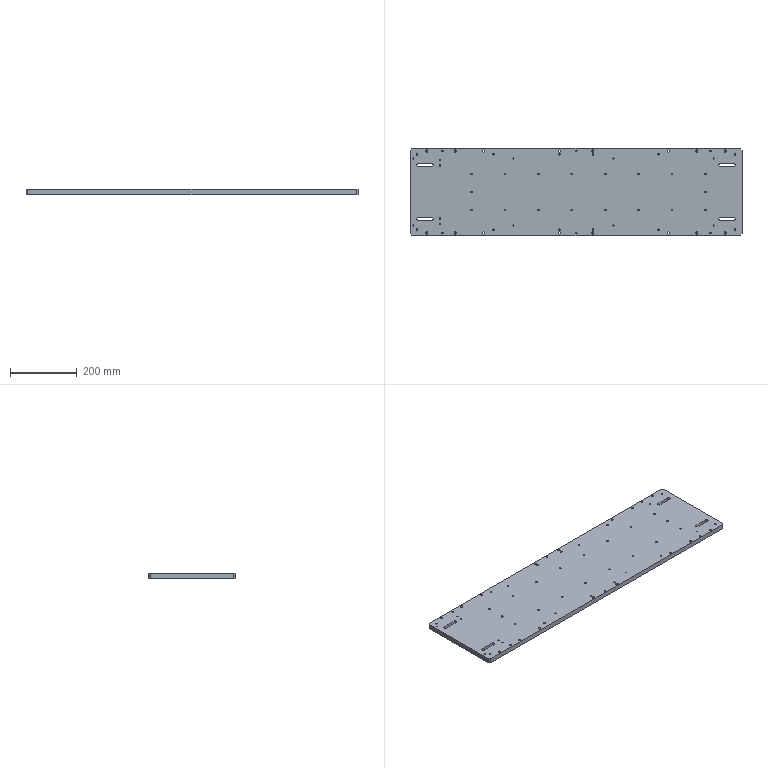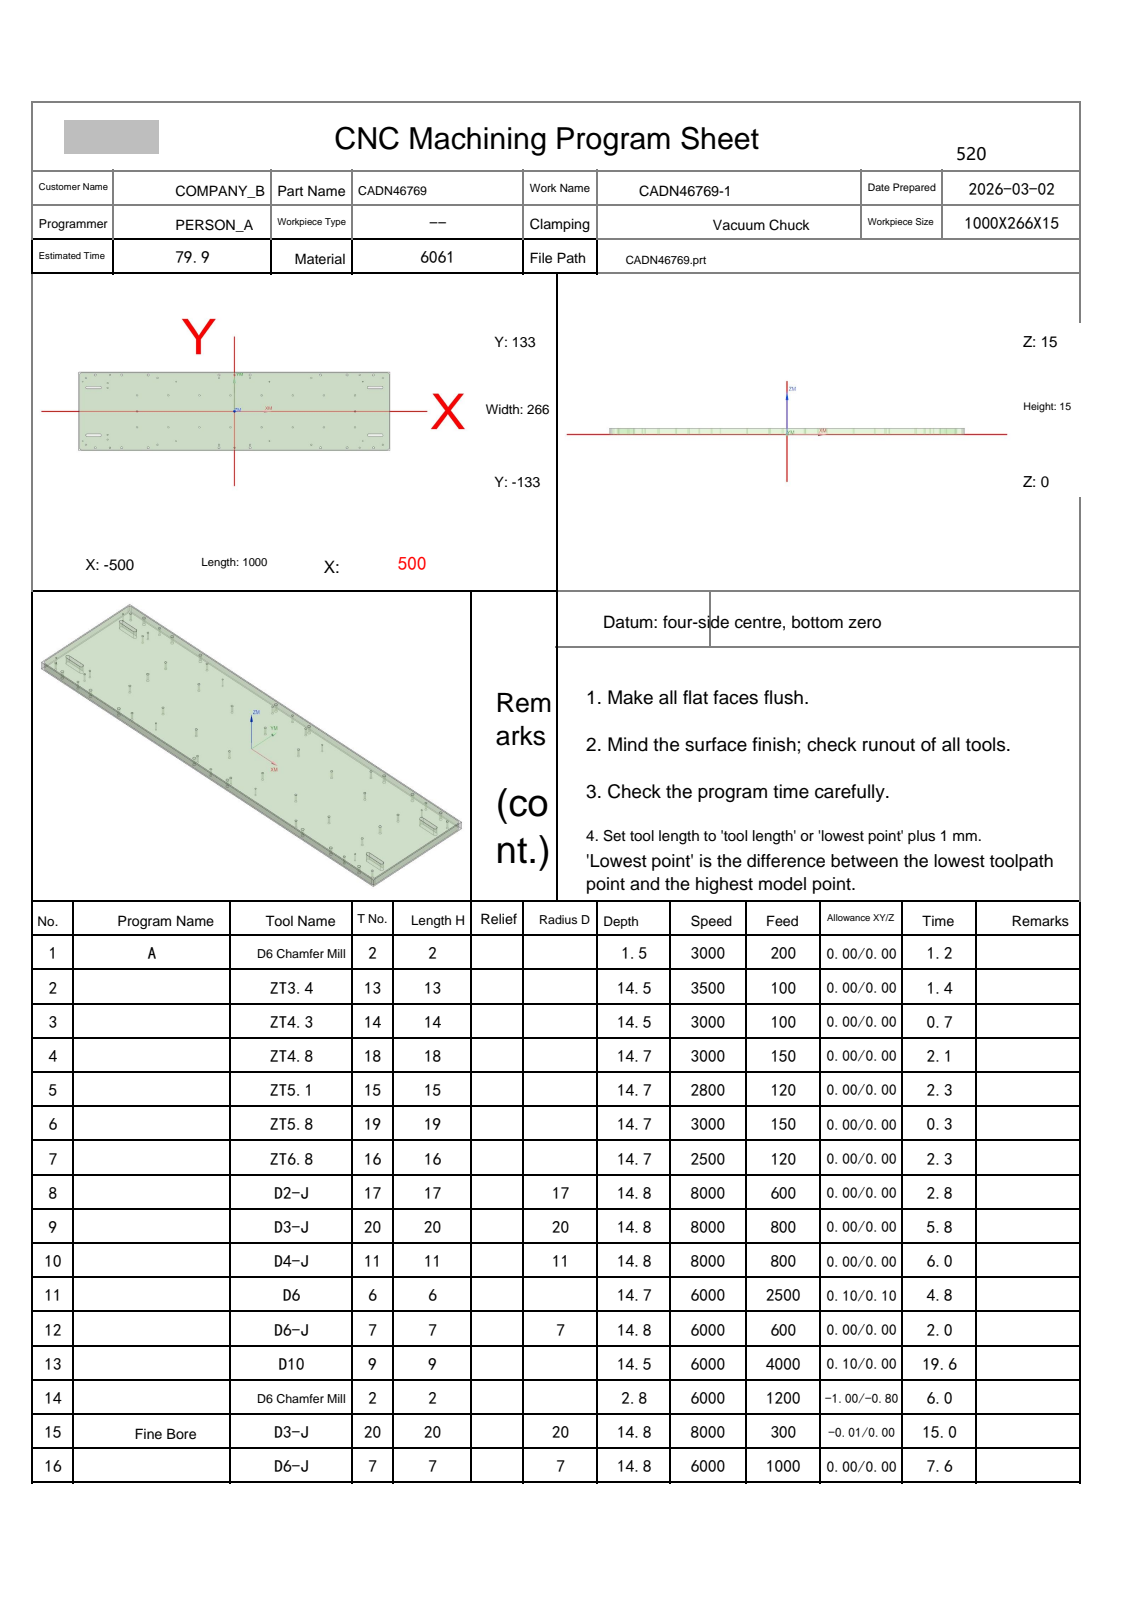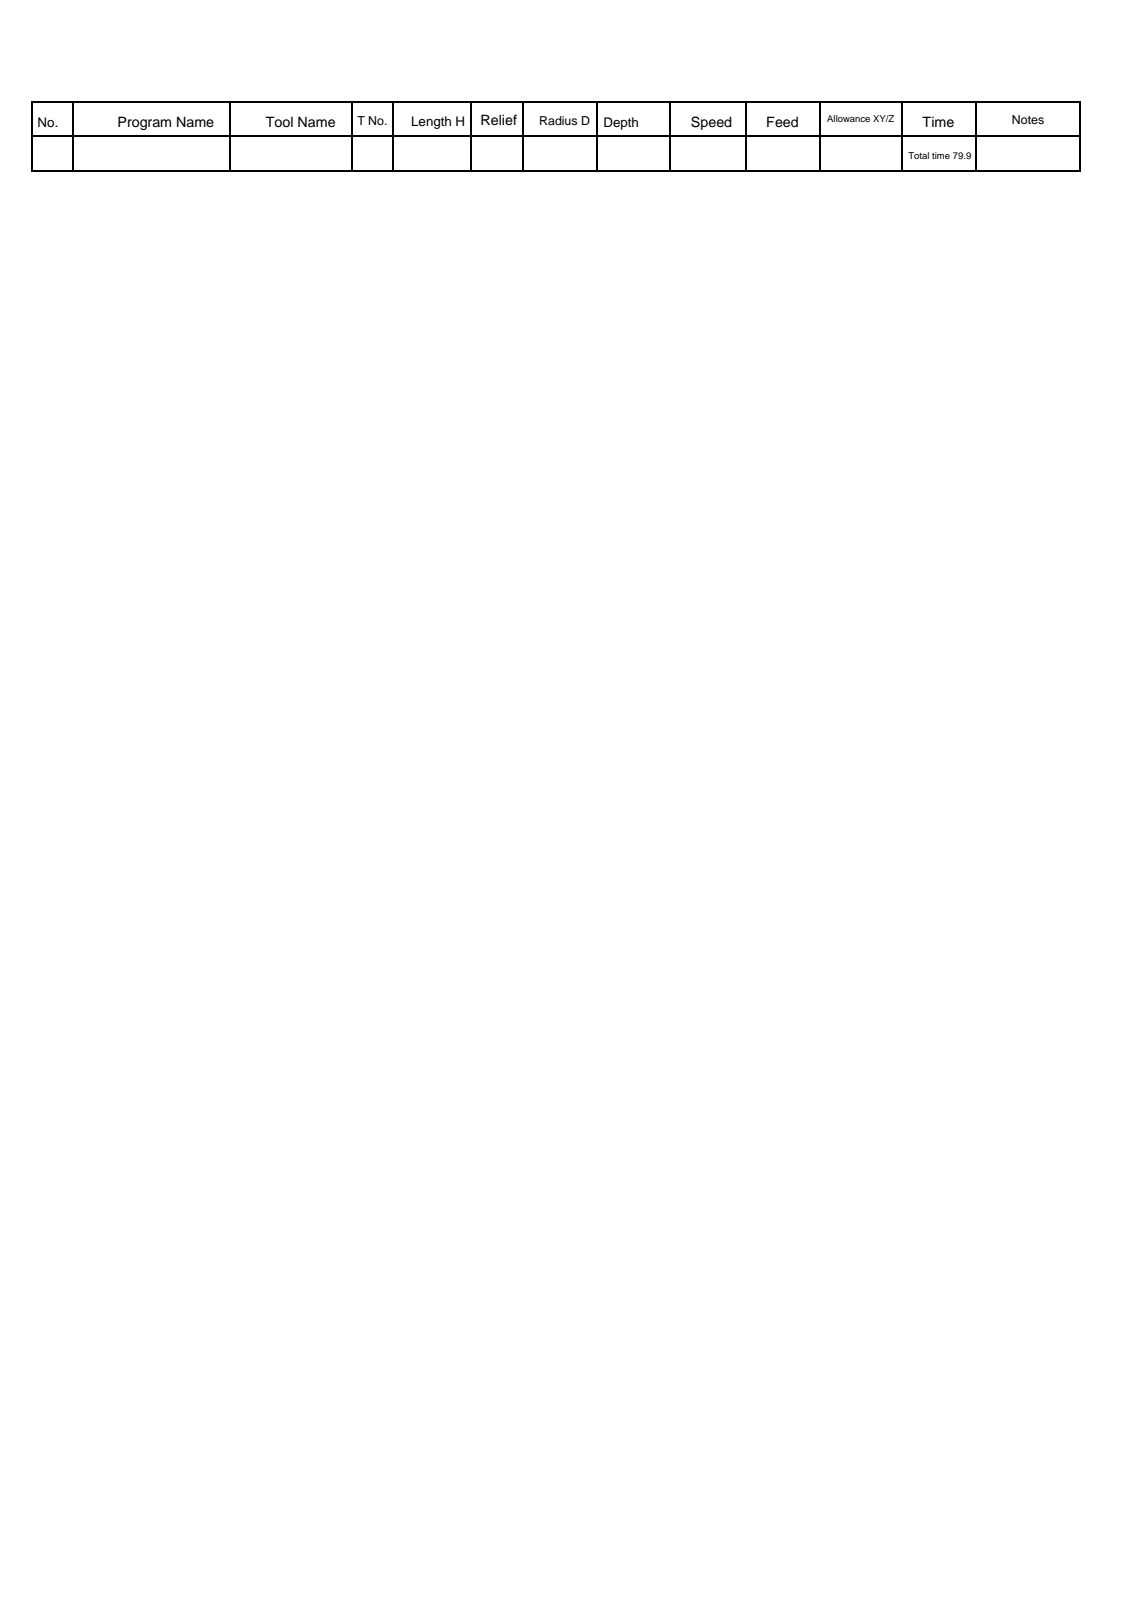NC program | NX | posted by the shop | part box 995 x 261 x 15 mm
Lines 2140 to 2975 of 14350:
N9 T20 M06
(D3-J  D=3. R=0. H=20 ce=0.00 di=0.00)
G00 G90 G54 X-407.387 Y-94.911 M03 S8000
G43 H20 Z45.
M08
Z15.5
G01 X-407.422 Y-94.9 Z15.498 F600.
X-407.578 Z15.49
X-407.767 Y-94.957 Z15.48
X-407.928 Y-95.072 Z15.469
X-408.043 Y-95.233 Z15.459
X-408.1 Y-95.422 Z15.448
Y-95.578 Z15.44
X-408.047 Y-95.758 Z15.43
X-407.941 Y-95.914 Z15.421
X-407.792 Y-96.03 Z15.411
X-407.615 Y-96.094 Z15.401
X-407.422 Y-96.1 Z15.391
X-407.233 Y-96.043 Z15.38
X-407.072 Y-95.928 Z15.37
X-406.957 Y-95.767 Z15.36
X-406.9 Y-95.578 Z15.349
Y-95.422 Z15.341
X-406.957 Y-95.233 Z15.331
X-407.072 Y-95.072 Z15.32
X-407.233 Y-94.957 Z15.31
X-407.422 Y-94.9 Z15.3
X-407.578 Z15.292
X-407.767 Y-94.957 Z15.281
X-407.928 Y-95.072 Z15.271
X-408.043 Y-95.233 Z15.26
X-408.1 Y-95.422 Z15.25
Y-95.578 Z15.242
X-408.047 Y-95.758 Z15.232
X-407.941 Y-95.914 Z15.222
X-407.792 Y-96.03 Z15.212
X-407.615 Y-96.094 Z15.202
X-407.422 Y-96.1 Z15.192
X-407.233 Y-96.043 Z15.182
X-407.072 Y-95.928 Z15.172
X-406.957 Y-95.767 Z15.161
X-406.9 Y-95.578 Z15.151
Y-95.422 Z15.143
X-406.957 Y-95.233 Z15.132
X-407.072 Y-95.072 Z15.122
X-407.233 Y-94.957 Z15.112
X-407.422 Y-94.9 Z15.101
X-407.578 Z15.093
X-407.767 Y-94.957 Z15.083
X-407.928 Y-95.072 Z15.072
X-408.043 Y-95.233 Z15.062
X-408.1 Y-95.422 Z15.052
Y-95.578 Z15.044
X-408.047 Y-95.758 Z15.034
X-407.941 Y-95.914 Z15.024
X-407.792 Y-96.03 Z15.014
X-407.615 Y-96.094 Z15.004
X-407.537 Y-96.099 Z15.
X-407.535 Y-96.065
G41 D20
X-407.5 Y-96.1
G03 X-406.9 Y-95.5 Z14.914 I0.0 J.6
X-407.5 Y-94.9 Z14.828 I-.6 J0.0
X-408.1 Y-95.5 Z14.742 I0.0 J-.6
X-407.5 Y-96.1 Z14.656 I.6 J0.0
X-406.9 Y-95.5 Z14.57 I0.0 J.6
X-407.5 Y-94.9 Z14.484 I-.6 J0.0
X-408.1 Y-95.5 Z14.398 I0.0 J-.6
X-407.5 Y-96.1 Z14.312 I.6 J0.0
X-406.9 Y-95.5 Z14.226 I0.0 J.6
X-407.5 Y-94.9 Z14.14 I-.6 J0.0
X-408.1 Y-95.5 Z14.053 I0.0 J-.6
X-407.5 Y-96.1 Z13.967 I.6 J0.0
X-406.9 Y-95.5 Z13.881 I0.0 J.6
X-407.5 Y-94.9 Z13.795 I-.6 J0.0
X-408.1 Y-95.5 Z13.709 I0.0 J-.6
X-407.5 Y-96.1 Z13.623 I.6 J0.0
X-406.9 Y-95.5 Z13.537 I0.0 J.6
X-407.5 Y-94.9 Z13.451 I-.6 J0.0
X-408.1 Y-95.5 Z13.365 I0.0 J-.6
X-407.5 Y-96.1 Z13.279 I.6 J0.0
X-406.9 Y-95.5 Z13.193 I0.0 J.6
X-407.5 Y-94.9 Z13.107 I-.6 J0.0
X-408.1 Y-95.5 Z13.021 I0.0 J-.6
X-407.5 Y-96.1 Z12.935 I.6 J0.0
X-406.9 Y-95.5 Z12.849 I0.0 J.6
X-407.5 Y-94.9 Z12.763 I-.6 J0.0
X-408.1 Y-95.5 Z12.677 I0.0 J-.6
X-407.5 Y-96.1 Z12.591 I.6 J0.0
X-406.9 Y-95.5 Z12.505 I0.0 J.6
X-407.5 Y-94.9 Z12.419 I-.6 J0.0
X-408.1 Y-95.5 Z12.333 I0.0 J-.6
X-407.5 Y-96.1 Z12.247 I.6 J0.0
X-406.9 Y-95.5 Z12.16 I0.0 J.6
X-407.5 Y-94.9 Z12.074 I-.6 J0.0
X-408.1 Y-95.5 Z11.988 I0.0 J-.6
X-407.5 Y-96.1 Z11.902 I.6 J0.0
X-406.9 Y-95.5 Z11.816 I0.0 J.6
X-407.5 Y-94.9 Z11.73 I-.6 J0.0
X-408.1 Y-95.5 Z11.644 I0.0 J-.6
X-407.5 Y-96.1 Z11.558 I.6 J0.0
X-406.9 Y-95.5 Z11.472 I0.0 J.6
X-407.5 Y-94.9 Z11.386 I-.6 J0.0
X-408.1 Y-95.5 Z11.3 I0.0 J-.6
X-407.5 Y-96.1 Z11.214 I.6 J0.0
X-406.9 Y-95.5 Z11.128 I0.0 J.6
X-407.5 Y-94.9 Z11.042 I-.6 J0.0
X-408.1 Y-95.5 Z10.956 I0.0 J-.6
X-407.5 Y-96.1 Z10.87 I.6 J0.0
X-406.9 Y-95.5 Z10.784 I0.0 J.6
X-407.5 Y-94.9 Z10.698 I-.6 J0.0
X-408.1 Y-95.5 Z10.612 I0.0 J-.6
X-407.5 Y-96.1 Z10.526 I.6 J0.0
X-406.9 Y-95.5 Z10.44 I0.0 J.6
X-407.5 Y-94.9 Z10.353 I-.6 J0.0
X-408.1 Y-95.5 Z10.267 I0.0 J-.6
X-407.5 Y-96.1 Z10.181 I.6 J0.0
X-406.9 Y-95.5 Z10.095 I0.0 J.6
X-407.5 Y-94.9 Z10.009 I-.6 J0.0
X-408.1 Y-95.5 Z9.923 I0.0 J-.6
X-407.5 Y-96.1 Z9.837 I.6 J0.0
X-406.9 Y-95.5 Z9.751 I0.0 J.6
X-407.5 Y-94.9 Z9.665 I-.6 J0.0
X-408.1 Y-95.5 Z9.579 I0.0 J-.6
X-407.5 Y-96.1 Z9.493 I.6 J0.0
X-406.9 Y-95.5 Z9.407 I0.0 J.6
X-407.5 Y-94.9 Z9.321 I-.6 J0.0
X-408.1 Y-95.5 Z9.235 I0.0 J-.6
X-407.5 Y-96.1 Z9.149 I.6 J0.0
X-406.9 Y-95.5 Z9.063 I0.0 J.6
X-407.5 Y-94.9 Z8.977 I-.6 J0.0
X-408.1 Y-95.5 Z8.891 I0.0 J-.6
X-407.5 Y-96.1 Z8.805 I.6 J0.0
X-406.9 Y-95.5 Z8.719 I0.0 J.6
X-407.5 Y-94.9 Z8.633 I-.6 J0.0
X-408.1 Y-95.5 Z8.547 I0.0 J-.6
X-407.5 Y-96.1 Z8.46 I.6 J0.0
X-406.9 Y-95.5 Z8.374 I0.0 J.6
X-407.5 Y-94.9 Z8.288 I-.6 J0.0
X-408.1 Y-95.5 Z8.202 I0.0 J-.6
X-407.5 Y-96.1 Z8.116 I.6 J0.0
X-406.9 Y-95.5 Z8.03 I0.0 J.6
X-407.5 Y-94.9 Z7.944 I-.6 J0.0
X-408.1 Y-95.5 Z7.858 I0.0 J-.6
X-407.5 Y-96.1 Z7.772 I.6 J0.0
X-406.9 Y-95.5 Z7.686 I0.0 J.6
X-407.5 Y-94.9 Z7.6 I-.6 J0.0
X-408.1 Y-95.5 Z7.514 I0.0 J-.6
X-407.5 Y-96.1 Z7.428 I.6 J0.0
X-406.9 Y-95.5 Z7.342 I0.0 J.6
X-407.5 Y-94.9 Z7.256 I-.6 J0.0
X-408.1 Y-95.5 Z7.17 I0.0 J-.6
X-407.5 Y-96.1 Z7.084 I.6 J0.0
X-406.9 Y-95.5 Z6.998 I0.0 J.6
X-407.5 Y-94.9 Z6.912 I-.6 J0.0
X-408.1 Y-95.5 Z6.826 I0.0 J-.6
X-407.5 Y-96.1 Z6.74 I.6 J0.0
X-406.9 Y-95.5 Z6.653 I0.0 J.6
X-407.5 Y-94.9 Z6.567 I-.6 J0.0
X-408.1 Y-95.5 Z6.481 I0.0 J-.6
X-407.5 Y-96.1 Z6.395 I.6 J0.0
X-406.9 Y-95.5 Z6.309 I0.0 J.6
X-407.5 Y-94.9 Z6.223 I-.6 J0.0
X-408.1 Y-95.5 Z6.137 I0.0 J-.6
X-407.5 Y-96.1 Z6.051 I.6 J0.0
X-406.9 Y-95.5 Z5.965 I0.0 J.6
X-407.5 Y-94.9 Z5.879 I-.6 J0.0
X-408.1 Y-95.5 Z5.793 I0.0 J-.6
X-407.5 Y-96.1 Z5.707 I.6 J0.0
X-406.9 Y-95.5 Z5.621 I0.0 J.6
X-407.5 Y-94.9 Z5.535 I-.6 J0.0
X-408.1 Y-95.5 Z5.449 I0.0 J-.6
X-407.5 Y-96.1 Z5.363 I.6 J0.0
X-406.9 Y-95.5 Z5.277 I0.0 J.6
X-407.5 Y-94.9 Z5.191 I-.6 J0.0
X-408.1 Y-95.5 Z5.105 I0.0 J-.6
X-407.5 Y-96.1 Z5.019 I.6 J0.0
X-406.9 Y-95.5 Z4.933 I0.0 J.6
X-407.5 Y-94.9 Z4.847 I-.6 J0.0
X-408.1 Y-95.5 Z4.76 I0.0 J-.6
X-407.5 Y-96.1 Z4.674 I.6 J0.0
X-406.9 Y-95.5 Z4.588 I0.0 J.6
X-407.5 Y-94.9 Z4.502 I-.6 J0.0
X-408.1 Y-95.5 Z4.416 I0.0 J-.6
X-407.5 Y-96.1 Z4.33 I.6 J0.0
X-406.9 Y-95.5 Z4.244 I0.0 J.6
X-407.5 Y-94.9 Z4.158 I-.6 J0.0
X-408.1 Y-95.5 Z4.072 I0.0 J-.6
X-407.5 Y-96.1 Z3.986 I.6 J0.0
X-406.9 Y-95.5 Z3.9 I0.0 J.6
X-407.5 Y-94.9 Z3.814 I-.6 J0.0
X-408.1 Y-95.5 Z3.728 I0.0 J-.6
X-407.5 Y-96.1 Z3.642 I.6 J0.0
X-406.9 Y-95.5 Z3.556 I0.0 J.6
X-407.5 Y-94.9 Z3.47 I-.6 J0.0
X-408.1 Y-95.5 Z3.384 I0.0 J-.6
X-407.5 Y-96.1 Z3.298 I.6 J0.0
X-406.9 Y-95.5 Z3.212 I0.0 J.6
X-407.5 Y-94.9 Z3.126 I-.6 J0.0
X-408.1 Y-95.5 Z3.04 I0.0 J-.6
X-407.5 Y-96.1 Z2.953 I.6 J0.0
X-406.9 Y-95.5 Z2.867 I0.0 J.6
X-407.5 Y-94.9 Z2.781 I-.6 J0.0
X-408.1 Y-95.5 Z2.695 I0.0 J-.6
X-407.5 Y-96.1 Z2.609 I.6 J0.0
X-406.9 Y-95.5 Z2.523 I0.0 J.6
X-407.5 Y-94.9 Z2.437 I-.6 J0.0
X-408.1 Y-95.5 Z2.351 I0.0 J-.6
X-407.5 Y-96.1 Z2.265 I.6 J0.0
X-406.9 Y-95.5 Z2.179 I0.0 J.6
X-407.5 Y-94.9 Z2.093 I-.6 J0.0
X-408.1 Y-95.5 Z2.007 I0.0 J-.6
X-407.5 Y-96.1 Z1.921 I.6 J0.0
X-406.9 Y-95.5 Z1.835 I0.0 J.6
X-407.5 Y-94.9 Z1.749 I-.6 J0.0
X-408.1 Y-95.5 Z1.663 I0.0 J-.6
X-407.5 Y-96.1 Z1.577 I.6 J0.0
X-406.9 Y-95.5 Z1.491 I0.0 J.6
X-407.5 Y-94.9 Z1.405 I-.6 J0.0
X-408.1 Y-95.5 Z1.319 I0.0 J-.6
X-407.5 Y-96.1 Z1.233 I.6 J0.0
X-406.9 Y-95.5 Z1.147 I0.0 J.6
X-407.5 Y-94.9 Z1.06 I-.6 J0.0
X-408.1 Y-95.5 Z.974 I0.0 J-.6
X-407.5 Y-96.1 Z.888 I.6 J0.0
X-406.9 Y-95.5 Z.802 I0.0 J.6
X-407.5 Y-94.9 Z.716 I-.6 J0.0
X-408.1 Y-95.5 Z.63 I0.0 J-.6
X-407.5 Y-96.1 Z.544 I.6 J0.0
X-406.9 Y-95.5 Z.458 I0.0 J.6
X-407.5 Y-94.9 Z.372 I-.6 J0.0
X-408.1 Y-95.5 Z.286 I0.0 J-.6
X-407.5 Y-96.1 Z.2 I.6 J0.0
X-406.9 Y-95.5 I0.0 J.6
X-407.5 Y-94.9 I-.6 J0.0
X-408.1 Y-95.5 I0.0 J-.6
X-407.5 Y-96.1 I.6 J0.0
X-407.129 Y-95.972 I0.0 J.6
G01 X-407.109 Y-95.953
X-407.105 Y-95.924
X-407.121 Y-95.901
G40 X-407.152 Y-95.862
Z1.2
G00 Z45.
X-407.387 Y-78.911
Z15.5
G01 X-407.422 Y-78.9 Z15.498
X-407.578 Z15.49
X-407.767 Y-78.957 Z15.48
X-407.928 Y-79.072 Z15.469
X-408.043 Y-79.233 Z15.459
X-408.1 Y-79.422 Z15.448
Y-79.578 Z15.44
X-408.047 Y-79.758 Z15.43
X-407.941 Y-79.914 Z15.421
X-407.792 Y-80.03 Z15.411
X-407.615 Y-80.094 Z15.401
X-407.422 Y-80.1 Z15.391
X-407.233 Y-80.043 Z15.38
X-407.072 Y-79.928 Z15.37
X-406.957 Y-79.767 Z15.36
X-406.9 Y-79.578 Z15.349
Y-79.422 Z15.341
X-406.957 Y-79.233 Z15.331
X-407.072 Y-79.072 Z15.32
X-407.233 Y-78.957 Z15.31
X-407.422 Y-78.9 Z15.3
X-407.578 Z15.292
X-407.767 Y-78.957 Z15.281
X-407.928 Y-79.072 Z15.271
X-408.043 Y-79.233 Z15.26
X-408.1 Y-79.422 Z15.25
Y-79.578 Z15.242
X-408.047 Y-79.758 Z15.232
X-407.941 Y-79.914 Z15.222
X-407.792 Y-80.03 Z15.212
X-407.615 Y-80.094 Z15.202
X-407.422 Y-80.1 Z15.192
X-407.233 Y-80.043 Z15.182
X-407.072 Y-79.928 Z15.172
X-406.957 Y-79.767 Z15.161
X-406.9 Y-79.578 Z15.151
Y-79.422 Z15.143
X-406.957 Y-79.233 Z15.132
X-407.072 Y-79.072 Z15.122
X-407.233 Y-78.957 Z15.112
X-407.422 Y-78.9 Z15.101
X-407.578 Z15.093
X-407.767 Y-78.957 Z15.083
X-407.928 Y-79.072 Z15.072
X-408.043 Y-79.233 Z15.062
X-408.1 Y-79.422 Z15.052
Y-79.578 Z15.044
X-408.047 Y-79.758 Z15.034
X-407.941 Y-79.914 Z15.024
X-407.792 Y-80.03 Z15.014
X-407.615 Y-80.094 Z15.004
X-407.537 Y-80.099 Z15.
X-407.535 Y-80.065
G41 D20
X-407.5 Y-80.1
G03 X-406.9 Y-79.5 Z14.914 I0.0 J.6
X-407.5 Y-78.9 Z14.828 I-.6 J0.0
X-408.1 Y-79.5 Z14.742 I0.0 J-.6
X-407.5 Y-80.1 Z14.656 I.6 J0.0
X-406.9 Y-79.5 Z14.57 I0.0 J.6
X-407.5 Y-78.9 Z14.484 I-.6 J0.0
X-408.1 Y-79.5 Z14.398 I0.0 J-.6
X-407.5 Y-80.1 Z14.312 I.6 J0.0
X-406.9 Y-79.5 Z14.226 I0.0 J.6
X-407.5 Y-78.9 Z14.14 I-.6 J0.0
X-408.1 Y-79.5 Z14.053 I0.0 J-.6
X-407.5 Y-80.1 Z13.967 I.6 J0.0
X-406.9 Y-79.5 Z13.881 I0.0 J.6
X-407.5 Y-78.9 Z13.795 I-.6 J0.0
X-408.1 Y-79.5 Z13.709 I0.0 J-.6
X-407.5 Y-80.1 Z13.623 I.6 J0.0
X-406.9 Y-79.5 Z13.537 I0.0 J.6
X-407.5 Y-78.9 Z13.451 I-.6 J0.0
X-408.1 Y-79.5 Z13.365 I0.0 J-.6
X-407.5 Y-80.1 Z13.279 I.6 J0.0
X-406.9 Y-79.5 Z13.193 I0.0 J.6
X-407.5 Y-78.9 Z13.107 I-.6 J0.0
X-408.1 Y-79.5 Z13.021 I0.0 J-.6
X-407.5 Y-80.1 Z12.935 I.6 J0.0
X-406.9 Y-79.5 Z12.849 I0.0 J.6
X-407.5 Y-78.9 Z12.763 I-.6 J0.0
X-408.1 Y-79.5 Z12.677 I0.0 J-.6
X-407.5 Y-80.1 Z12.591 I.6 J0.0
X-406.9 Y-79.5 Z12.505 I0.0 J.6
X-407.5 Y-78.9 Z12.419 I-.6 J0.0
X-408.1 Y-79.5 Z12.333 I0.0 J-.6
X-407.5 Y-80.1 Z12.247 I.6 J0.0
X-406.9 Y-79.5 Z12.16 I0.0 J.6
X-407.5 Y-78.9 Z12.074 I-.6 J0.0
X-408.1 Y-79.5 Z11.988 I0.0 J-.6
X-407.5 Y-80.1 Z11.902 I.6 J0.0
X-406.9 Y-79.5 Z11.816 I0.0 J.6
X-407.5 Y-78.9 Z11.73 I-.6 J0.0
X-408.1 Y-79.5 Z11.644 I0.0 J-.6
X-407.5 Y-80.1 Z11.558 I.6 J0.0
X-406.9 Y-79.5 Z11.472 I0.0 J.6
X-407.5 Y-78.9 Z11.386 I-.6 J0.0
X-408.1 Y-79.5 Z11.3 I0.0 J-.6
X-407.5 Y-80.1 Z11.214 I.6 J0.0
X-406.9 Y-79.5 Z11.128 I0.0 J.6
X-407.5 Y-78.9 Z11.042 I-.6 J0.0
X-408.1 Y-79.5 Z10.956 I0.0 J-.6
X-407.5 Y-80.1 Z10.87 I.6 J0.0
X-406.9 Y-79.5 Z10.784 I0.0 J.6
X-407.5 Y-78.9 Z10.698 I-.6 J0.0
X-408.1 Y-79.5 Z10.612 I0.0 J-.6
X-407.5 Y-80.1 Z10.526 I.6 J0.0
X-406.9 Y-79.5 Z10.44 I0.0 J.6
X-407.5 Y-78.9 Z10.353 I-.6 J0.0
X-408.1 Y-79.5 Z10.267 I0.0 J-.6
X-407.5 Y-80.1 Z10.181 I.6 J0.0
X-406.9 Y-79.5 Z10.095 I0.0 J.6
X-407.5 Y-78.9 Z10.009 I-.6 J0.0
X-408.1 Y-79.5 Z9.923 I0.0 J-.6
X-407.5 Y-80.1 Z9.837 I.6 J0.0
X-406.9 Y-79.5 Z9.751 I0.0 J.6
X-407.5 Y-78.9 Z9.665 I-.6 J0.0
X-408.1 Y-79.5 Z9.579 I0.0 J-.6
X-407.5 Y-80.1 Z9.493 I.6 J0.0
X-406.9 Y-79.5 Z9.407 I0.0 J.6
X-407.5 Y-78.9 Z9.321 I-.6 J0.0
X-408.1 Y-79.5 Z9.235 I0.0 J-.6
X-407.5 Y-80.1 Z9.149 I.6 J0.0
X-406.9 Y-79.5 Z9.063 I0.0 J.6
X-407.5 Y-78.9 Z8.977 I-.6 J0.0
X-408.1 Y-79.5 Z8.891 I0.0 J-.6
X-407.5 Y-80.1 Z8.805 I.6 J0.0
X-406.9 Y-79.5 Z8.719 I0.0 J.6
X-407.5 Y-78.9 Z8.633 I-.6 J0.0
X-408.1 Y-79.5 Z8.547 I0.0 J-.6
X-407.5 Y-80.1 Z8.46 I.6 J0.0
X-406.9 Y-79.5 Z8.374 I0.0 J.6
X-407.5 Y-78.9 Z8.288 I-.6 J0.0
X-408.1 Y-79.5 Z8.202 I0.0 J-.6
X-407.5 Y-80.1 Z8.116 I.6 J0.0
X-406.9 Y-79.5 Z8.03 I0.0 J.6
X-407.5 Y-78.9 Z7.944 I-.6 J0.0
X-408.1 Y-79.5 Z7.858 I0.0 J-.6
X-407.5 Y-80.1 Z7.772 I.6 J0.0
X-406.9 Y-79.5 Z7.686 I0.0 J.6
X-407.5 Y-78.9 Z7.6 I-.6 J0.0
X-408.1 Y-79.5 Z7.514 I0.0 J-.6
X-407.5 Y-80.1 Z7.428 I.6 J0.0
X-406.9 Y-79.5 Z7.342 I0.0 J.6
X-407.5 Y-78.9 Z7.256 I-.6 J0.0
X-408.1 Y-79.5 Z7.17 I0.0 J-.6
X-407.5 Y-80.1 Z7.084 I.6 J0.0
X-406.9 Y-79.5 Z6.998 I0.0 J.6
X-407.5 Y-78.9 Z6.912 I-.6 J0.0
X-408.1 Y-79.5 Z6.826 I0.0 J-.6
X-407.5 Y-80.1 Z6.74 I.6 J0.0
X-406.9 Y-79.5 Z6.653 I0.0 J.6
X-407.5 Y-78.9 Z6.567 I-.6 J0.0
X-408.1 Y-79.5 Z6.481 I0.0 J-.6
X-407.5 Y-80.1 Z6.395 I.6 J0.0
X-406.9 Y-79.5 Z6.309 I0.0 J.6
X-407.5 Y-78.9 Z6.223 I-.6 J0.0
X-408.1 Y-79.5 Z6.137 I0.0 J-.6
X-407.5 Y-80.1 Z6.051 I.6 J0.0
X-406.9 Y-79.5 Z5.965 I0.0 J.6
X-407.5 Y-78.9 Z5.879 I-.6 J0.0
X-408.1 Y-79.5 Z5.793 I0.0 J-.6
X-407.5 Y-80.1 Z5.707 I.6 J0.0
X-406.9 Y-79.5 Z5.621 I0.0 J.6
X-407.5 Y-78.9 Z5.535 I-.6 J0.0
X-408.1 Y-79.5 Z5.449 I0.0 J-.6
X-407.5 Y-80.1 Z5.363 I.6 J0.0
X-406.9 Y-79.5 Z5.277 I0.0 J.6
X-407.5 Y-78.9 Z5.191 I-.6 J0.0
X-408.1 Y-79.5 Z5.105 I0.0 J-.6
X-407.5 Y-80.1 Z5.019 I.6 J0.0
X-406.9 Y-79.5 Z4.933 I0.0 J.6
X-407.5 Y-78.9 Z4.847 I-.6 J0.0
X-408.1 Y-79.5 Z4.76 I0.0 J-.6
X-407.5 Y-80.1 Z4.674 I.6 J0.0
X-406.9 Y-79.5 Z4.588 I0.0 J.6
X-407.5 Y-78.9 Z4.502 I-.6 J0.0
X-408.1 Y-79.5 Z4.416 I0.0 J-.6
X-407.5 Y-80.1 Z4.33 I.6 J0.0
X-406.9 Y-79.5 Z4.244 I0.0 J.6
X-407.5 Y-78.9 Z4.158 I-.6 J0.0
X-408.1 Y-79.5 Z4.072 I0.0 J-.6
X-407.5 Y-80.1 Z3.986 I.6 J0.0
X-406.9 Y-79.5 Z3.9 I0.0 J.6
X-407.5 Y-78.9 Z3.814 I-.6 J0.0
X-408.1 Y-79.5 Z3.728 I0.0 J-.6
X-407.5 Y-80.1 Z3.642 I.6 J0.0
X-406.9 Y-79.5 Z3.556 I0.0 J.6
X-407.5 Y-78.9 Z3.47 I-.6 J0.0
X-408.1 Y-79.5 Z3.384 I0.0 J-.6
X-407.5 Y-80.1 Z3.298 I.6 J0.0
X-406.9 Y-79.5 Z3.212 I0.0 J.6
X-407.5 Y-78.9 Z3.126 I-.6 J0.0
X-408.1 Y-79.5 Z3.04 I0.0 J-.6
X-407.5 Y-80.1 Z2.953 I.6 J0.0
X-406.9 Y-79.5 Z2.867 I0.0 J.6
X-407.5 Y-78.9 Z2.781 I-.6 J0.0
X-408.1 Y-79.5 Z2.695 I0.0 J-.6
X-407.5 Y-80.1 Z2.609 I.6 J0.0
X-406.9 Y-79.5 Z2.523 I0.0 J.6
X-407.5 Y-78.9 Z2.437 I-.6 J0.0
X-408.1 Y-79.5 Z2.351 I0.0 J-.6
X-407.5 Y-80.1 Z2.265 I.6 J0.0
X-406.9 Y-79.5 Z2.179 I0.0 J.6
X-407.5 Y-78.9 Z2.093 I-.6 J0.0
X-408.1 Y-79.5 Z2.007 I0.0 J-.6
X-407.5 Y-80.1 Z1.921 I.6 J0.0
X-406.9 Y-79.5 Z1.835 I0.0 J.6
X-407.5 Y-78.9 Z1.749 I-.6 J0.0
X-408.1 Y-79.5 Z1.663 I0.0 J-.6
X-407.5 Y-80.1 Z1.577 I.6 J0.0
X-406.9 Y-79.5 Z1.491 I0.0 J.6
X-407.5 Y-78.9 Z1.405 I-.6 J0.0
X-408.1 Y-79.5 Z1.319 I0.0 J-.6
X-407.5 Y-80.1 Z1.233 I.6 J0.0
X-406.9 Y-79.5 Z1.147 I0.0 J.6
X-407.5 Y-78.9 Z1.06 I-.6 J0.0
X-408.1 Y-79.5 Z.974 I0.0 J-.6
X-407.5 Y-80.1 Z.888 I.6 J0.0
X-406.9 Y-79.5 Z.802 I0.0 J.6
X-407.5 Y-78.9 Z.716 I-.6 J0.0
X-408.1 Y-79.5 Z.63 I0.0 J-.6
X-407.5 Y-80.1 Z.544 I.6 J0.0
X-406.9 Y-79.5 Z.458 I0.0 J.6
X-407.5 Y-78.9 Z.372 I-.6 J0.0
X-408.1 Y-79.5 Z.286 I0.0 J-.6
X-407.5 Y-80.1 Z.2 I.6 J0.0
X-406.9 Y-79.5 I0.0 J.6
X-407.5 Y-78.9 I-.6 J0.0
X-408.1 Y-79.5 I0.0 J-.6
X-407.5 Y-80.1 I.6 J0.0
X-407.129 Y-79.972 I0.0 J.6
G01 X-407.109 Y-79.953
X-407.105 Y-79.924
X-407.121 Y-79.901
G40 X-407.152 Y-79.862
Z1.2
G00 Z45.
X-407.613 Y78.911
Z15.5
G01 X-407.578 Y78.9 Z15.498
X-407.422 Z15.49
X-407.233 Y78.957 Z15.48
X-407.072 Y79.072 Z15.469
X-406.957 Y79.233 Z15.459
X-406.9 Y79.422 Z15.448
Y79.578 Z15.44
X-406.953 Y79.758 Z15.43
X-407.059 Y79.914 Z15.421
X-407.208 Y80.03 Z15.411
X-407.385 Y80.094 Z15.401
X-407.578 Y80.1 Z15.391
X-407.767 Y80.043 Z15.38
X-407.928 Y79.928 Z15.37
X-408.043 Y79.767 Z15.36
X-408.1 Y79.578 Z15.349
Y79.422 Z15.341
X-408.043 Y79.233 Z15.331
X-407.928 Y79.072 Z15.32
X-407.767 Y78.957 Z15.31
X-407.578 Y78.9 Z15.3
X-407.422 Z15.292
X-407.233 Y78.957 Z15.281
X-407.072 Y79.072 Z15.271
X-406.957 Y79.233 Z15.26
X-406.9 Y79.422 Z15.25
Y79.578 Z15.242
X-406.953 Y79.758 Z15.232
X-407.059 Y79.914 Z15.222
X-407.208 Y80.03 Z15.212
X-407.385 Y80.094 Z15.202
X-407.578 Y80.1 Z15.192
X-407.767 Y80.043 Z15.182
X-407.928 Y79.928 Z15.172
X-408.043 Y79.767 Z15.161
X-408.1 Y79.578 Z15.151
Y79.422 Z15.143
X-408.043 Y79.233 Z15.132
X-407.928 Y79.072 Z15.122
X-407.767 Y78.957 Z15.112
X-407.578 Y78.9 Z15.101
X-407.422 Z15.093
X-407.233 Y78.957 Z15.083
X-407.072 Y79.072 Z15.072
X-406.957 Y79.233 Z15.062
X-406.9 Y79.422 Z15.052
Y79.578 Z15.044
X-406.953 Y79.758 Z15.034
X-407.059 Y79.914 Z15.024
X-407.208 Y80.03 Z15.014
X-407.385 Y80.094 Z15.004
X-407.463 Y80.099 Z15.
X-407.465 Y80.065
G41 D20
X-407.5 Y80.1
G03 X-408.1 Y79.5 Z14.914 I0.0 J-.6
X-407.5 Y78.9 Z14.828 I.6 J0.0
X-406.9 Y79.5 Z14.742 I0.0 J.6
X-407.5 Y80.1 Z14.656 I-.6 J0.0
X-408.1 Y79.5 Z14.57 I0.0 J-.6
X-407.5 Y78.9 Z14.484 I.6 J0.0
X-406.9 Y79.5 Z14.398 I0.0 J.6
X-407.5 Y80.1 Z14.312 I-.6 J0.0
X-408.1 Y79.5 Z14.226 I0.0 J-.6
X-407.5 Y78.9 Z14.14 I.6 J0.0
X-406.9 Y79.5 Z14.053 I0.0 J.6
X-407.5 Y80.1 Z13.967 I-.6 J0.0
X-408.1 Y79.5 Z13.881 I0.0 J-.6
X-407.5 Y78.9 Z13.795 I.6 J0.0
X-406.9 Y79.5 Z13.709 I0.0 J.6
X-407.5 Y80.1 Z13.623 I-.6 J0.0
X-408.1 Y79.5 Z13.537 I0.0 J-.6
X-407.5 Y78.9 Z13.451 I.6 J0.0
X-406.9 Y79.5 Z13.365 I0.0 J.6
X-407.5 Y80.1 Z13.279 I-.6 J0.0
X-408.1 Y79.5 Z13.193 I0.0 J-.6
X-407.5 Y78.9 Z13.107 I.6 J0.0
X-406.9 Y79.5 Z13.021 I0.0 J.6
X-407.5 Y80.1 Z12.935 I-.6 J0.0
X-408.1 Y79.5 Z12.849 I0.0 J-.6
X-407.5 Y78.9 Z12.763 I.6 J0.0
X-406.9 Y79.5 Z12.677 I0.0 J.6
X-407.5 Y80.1 Z12.591 I-.6 J0.0
X-408.1 Y79.5 Z12.505 I0.0 J-.6
X-407.5 Y78.9 Z12.419 I.6 J0.0
X-406.9 Y79.5 Z12.333 I0.0 J.6
X-407.5 Y80.1 Z12.247 I-.6 J0.0
X-408.1 Y79.5 Z12.16 I0.0 J-.6
X-407.5 Y78.9 Z12.074 I.6 J0.0
X-406.9 Y79.5 Z11.988 I0.0 J.6
X-407.5 Y80.1 Z11.902 I-.6 J0.0
X-408.1 Y79.5 Z11.816 I0.0 J-.6
X-407.5 Y78.9 Z11.73 I.6 J0.0
X-406.9 Y79.5 Z11.644 I0.0 J.6
X-407.5 Y80.1 Z11.558 I-.6 J0.0
X-408.1 Y79.5 Z11.472 I0.0 J-.6
X-407.5 Y78.9 Z11.386 I.6 J0.0
X-406.9 Y79.5 Z11.3 I0.0 J.6
X-407.5 Y80.1 Z11.214 I-.6 J0.0
X-408.1 Y79.5 Z11.128 I0.0 J-.6
X-407.5 Y78.9 Z11.042 I.6 J0.0
X-406.9 Y79.5 Z10.956 I0.0 J.6
X-407.5 Y80.1 Z10.87 I-.6 J0.0
X-408.1 Y79.5 Z10.784 I0.0 J-.6
X-407.5 Y78.9 Z10.698 I.6 J0.0
X-406.9 Y79.5 Z10.612 I0.0 J.6
X-407.5 Y80.1 Z10.526 I-.6 J0.0
X-408.1 Y79.5 Z10.44 I0.0 J-.6
X-407.5 Y78.9 Z10.353 I.6 J0.0
X-406.9 Y79.5 Z10.267 I0.0 J.6
X-407.5 Y80.1 Z10.181 I-.6 J0.0
X-408.1 Y79.5 Z10.095 I0.0 J-.6
X-407.5 Y78.9 Z10.009 I.6 J0.0
X-406.9 Y79.5 Z9.923 I0.0 J.6
X-407.5 Y80.1 Z9.837 I-.6 J0.0
X-408.1 Y79.5 Z9.751 I0.0 J-.6
X-407.5 Y78.9 Z9.665 I.6 J0.0
X-406.9 Y79.5 Z9.579 I0.0 J.6
X-407.5 Y80.1 Z9.493 I-.6 J0.0
X-408.1 Y79.5 Z9.407 I0.0 J-.6
X-407.5 Y78.9 Z9.321 I.6 J0.0
X-406.9 Y79.5 Z9.235 I0.0 J.6
X-407.5 Y80.1 Z9.149 I-.6 J0.0
X-408.1 Y79.5 Z9.063 I0.0 J-.6
X-407.5 Y78.9 Z8.977 I.6 J0.0
X-406.9 Y79.5 Z8.891 I0.0 J.6
X-407.5 Y80.1 Z8.805 I-.6 J0.0
X-408.1 Y79.5 Z8.719 I0.0 J-.6
X-407.5 Y78.9 Z8.633 I.6 J0.0
X-406.9 Y79.5 Z8.547 I0.0 J.6
X-407.5 Y80.1 Z8.46 I-.6 J0.0
X-408.1 Y79.5 Z8.374 I0.0 J-.6
X-407.5 Y78.9 Z8.288 I.6 J0.0
X-406.9 Y79.5 Z8.202 I0.0 J.6
X-407.5 Y80.1 Z8.116 I-.6 J0.0
X-408.1 Y79.5 Z8.03 I0.0 J-.6
X-407.5 Y78.9 Z7.944 I.6 J0.0
X-406.9 Y79.5 Z7.858 I0.0 J.6
X-407.5 Y80.1 Z7.772 I-.6 J0.0
X-408.1 Y79.5 Z7.686 I0.0 J-.6
X-407.5 Y78.9 Z7.6 I.6 J0.0
X-406.9 Y79.5 Z7.514 I0.0 J.6
X-407.5 Y80.1 Z7.428 I-.6 J0.0
X-408.1 Y79.5 Z7.342 I0.0 J-.6
X-407.5 Y78.9 Z7.256 I.6 J0.0
X-406.9 Y79.5 Z7.17 I0.0 J.6
X-407.5 Y80.1 Z7.084 I-.6 J0.0
X-408.1 Y79.5 Z6.998 I0.0 J-.6
X-407.5 Y78.9 Z6.912 I.6 J0.0
X-406.9 Y79.5 Z6.826 I0.0 J.6
X-407.5 Y80.1 Z6.74 I-.6 J0.0
X-408.1 Y79.5 Z6.653 I0.0 J-.6
X-407.5 Y78.9 Z6.567 I.6 J0.0
X-406.9 Y79.5 Z6.481 I0.0 J.6
X-407.5 Y80.1 Z6.395 I-.6 J0.0
X-408.1 Y79.5 Z6.309 I0.0 J-.6
X-407.5 Y78.9 Z6.223 I.6 J0.0
X-406.9 Y79.5 Z6.137 I0.0 J.6
X-407.5 Y80.1 Z6.051 I-.6 J0.0
X-408.1 Y79.5 Z5.965 I0.0 J-.6
X-407.5 Y78.9 Z5.879 I.6 J0.0
X-406.9 Y79.5 Z5.793 I0.0 J.6
X-407.5 Y80.1 Z5.707 I-.6 J0.0
X-408.1 Y79.5 Z5.621 I0.0 J-.6
X-407.5 Y78.9 Z5.535 I.6 J0.0
X-406.9 Y79.5 Z5.449 I0.0 J.6
X-407.5 Y80.1 Z5.363 I-.6 J0.0
X-408.1 Y79.5 Z5.277 I0.0 J-.6
X-407.5 Y78.9 Z5.191 I.6 J0.0
X-406.9 Y79.5 Z5.105 I0.0 J.6
X-407.5 Y80.1 Z5.019 I-.6 J0.0
X-408.1 Y79.5 Z4.933 I0.0 J-.6
X-407.5 Y78.9 Z4.847 I.6 J0.0
X-406.9 Y79.5 Z4.76 I0.0 J.6
X-407.5 Y80.1 Z4.674 I-.6 J0.0
X-408.1 Y79.5 Z4.588 I0.0 J-.6
X-407.5 Y78.9 Z4.502 I.6 J0.0
X-406.9 Y79.5 Z4.416 I0.0 J.6
X-407.5 Y80.1 Z4.33 I-.6 J0.0
X-408.1 Y79.5 Z4.244 I0.0 J-.6
X-407.5 Y78.9 Z4.158 I.6 J0.0
X-406.9 Y79.5 Z4.072 I0.0 J.6
X-407.5 Y80.1 Z3.986 I-.6 J0.0
X-408.1 Y79.5 Z3.9 I0.0 J-.6
X-407.5 Y78.9 Z3.814 I.6 J0.0
X-406.9 Y79.5 Z3.728 I0.0 J.6
X-407.5 Y80.1 Z3.642 I-.6 J0.0
X-408.1 Y79.5 Z3.556 I0.0 J-.6
X-407.5 Y78.9 Z3.47 I.6 J0.0
X-406.9 Y79.5 Z3.384 I0.0 J.6
X-407.5 Y80.1 Z3.298 I-.6 J0.0
X-408.1 Y79.5 Z3.212 I0.0 J-.6
X-407.5 Y78.9 Z3.126 I.6 J0.0
X-406.9 Y79.5 Z3.04 I0.0 J.6
X-407.5 Y80.1 Z2.953 I-.6 J0.0
X-408.1 Y79.5 Z2.867 I0.0 J-.6
X-407.5 Y78.9 Z2.781 I.6 J0.0
X-406.9 Y79.5 Z2.695 I0.0 J.6
X-407.5 Y80.1 Z2.609 I-.6 J0.0
X-408.1 Y79.5 Z2.523 I0.0 J-.6
X-407.5 Y78.9 Z2.437 I.6 J0.0
X-406.9 Y79.5 Z2.351 I0.0 J.6
X-407.5 Y80.1 Z2.265 I-.6 J0.0
X-408.1 Y79.5 Z2.179 I0.0 J-.6
X-407.5 Y78.9 Z2.093 I.6 J0.0
X-406.9 Y79.5 Z2.007 I0.0 J.6
X-407.5 Y80.1 Z1.921 I-.6 J0.0
X-408.1 Y79.5 Z1.835 I0.0 J-.6
X-407.5 Y78.9 Z1.749 I.6 J0.0
X-406.9 Y79.5 Z1.663 I0.0 J.6
X-407.5 Y80.1 Z1.577 I-.6 J0.0
X-408.1 Y79.5 Z1.491 I0.0 J-.6
X-407.5 Y78.9 Z1.405 I.6 J0.0
X-406.9 Y79.5 Z1.319 I0.0 J.6
X-407.5 Y80.1 Z1.233 I-.6 J0.0
X-408.1 Y79.5 Z1.147 I0.0 J-.6
X-407.5 Y78.9 Z1.06 I.6 J0.0
X-406.9 Y79.5 Z.974 I0.0 J.6
X-407.5 Y80.1 Z.888 I-.6 J0.0
X-408.1 Y79.5 Z.802 I0.0 J-.6
X-407.5 Y78.9 Z.716 I.6 J0.0
X-406.9 Y79.5 Z.63 I0.0 J.6
X-407.5 Y80.1 Z.544 I-.6 J0.0
X-408.1 Y79.5 Z.458 I0.0 J-.6
X-407.5 Y78.9 Z.372 I.6 J0.0
X-406.9 Y79.5 Z.286 I0.0 J.6
X-407.5 Y80.1 Z.2 I-.6 J0.0
X-408.1 Y79.5 I0.0 J-.6
X-407.5 Y78.9 I.6 J0.0
X-406.9 Y79.5 I0.0 J.6
X-407.5 Y80.1 I-.6 J0.0
X-407.871 Y79.972 I0.0 J-.6
G01 X-407.891 Y79.953
X-407.895 Y79.924
X-407.879 Y79.901
G40 X-407.848 Y79.862
Z1.2
G00 Z45.
X-407.613 Y94.911
Z15.5
G01 X-407.578 Y94.9 Z15.498
X-407.422 Z15.49
X-407.233 Y94.957 Z15.48
X-407.072 Y95.072 Z15.469
X-406.957 Y95.233 Z15.459
X-406.9 Y95.422 Z15.448
Y95.578 Z15.44
X-406.953 Y95.758 Z15.43
X-407.059 Y95.914 Z15.421
X-407.208 Y96.03 Z15.411
X-407.385 Y96.094 Z15.401
X-407.578 Y96.1 Z15.391
X-407.767 Y96.043 Z15.38
X-407.928 Y95.928 Z15.37
X-408.043 Y95.767 Z15.36
X-408.1 Y95.578 Z15.349
Y95.422 Z15.341
X-408.043 Y95.233 Z15.331
X-407.928 Y95.072 Z15.32
X-407.767 Y94.957 Z15.31
X-407.578 Y94.9 Z15.3
X-407.422 Z15.292
X-407.233 Y94.957 Z15.281
X-407.072 Y95.072 Z15.271
X-406.957 Y95.233 Z15.26
X-406.9 Y95.422 Z15.25
Y95.578 Z15.242
X-406.953 Y95.758 Z15.232
X-407.059 Y95.914 Z15.222
X-407.208 Y96.03 Z15.212
X-407.385 Y96.094 Z15.202
X-407.578 Y96.1 Z15.192
X-407.767 Y96.043 Z15.182
X-407.928 Y95.928 Z15.172
X-408.043 Y95.767 Z15.161
X-408.1 Y95.578 Z15.151
Y95.422 Z15.143
X-408.043 Y95.233 Z15.132
X-407.928 Y95.072 Z15.122
X-407.767 Y94.957 Z15.112
X-407.578 Y94.9 Z15.101
X-407.422 Z15.093
X-407.233 Y94.957 Z15.083
X-407.072 Y95.072 Z15.072
X-406.957 Y95.233 Z15.062
X-406.9 Y95.422 Z15.052
Y95.578 Z15.044
X-406.953 Y95.758 Z15.034
X-407.059 Y95.914 Z15.024
X-407.208 Y96.03 Z15.014
X-407.385 Y96.094 Z15.004
X-407.463 Y96.099 Z15.
X-407.465 Y96.065
G41 D20
X-407.5 Y96.1
G03 X-408.1 Y95.5 Z14.914 I0.0 J-.6
X-407.5 Y94.9 Z14.828 I.6 J0.0
X-406.9 Y95.5 Z14.742 I0.0 J.6
X-407.5 Y96.1 Z14.656 I-.6 J0.0
X-408.1 Y95.5 Z14.57 I0.0 J-.6
X-407.5 Y94.9 Z14.484 I.6 J0.0
X-406.9 Y95.5 Z14.398 I0.0 J.6
X-407.5 Y96.1 Z14.312 I-.6 J0.0
X-408.1 Y95.5 Z14.226 I0.0 J-.6
X-407.5 Y94.9 Z14.14 I.6 J0.0
X-406.9 Y95.5 Z14.053 I0.0 J.6
X-407.5 Y96.1 Z13.967 I-.6 J0.0
X-408.1 Y95.5 Z13.881 I0.0 J-.6
X-407.5 Y94.9 Z13.795 I.6 J0.0
X-406.9 Y95.5 Z13.709 I0.0 J.6
X-407.5 Y96.1 Z13.623 I-.6 J0.0
X-408.1 Y95.5 Z13.537 I0.0 J-.6
X-407.5 Y94.9 Z13.451 I.6 J0.0
X-406.9 Y95.5 Z13.365 I0.0 J.6
X-407.5 Y96.1 Z13.279 I-.6 J0.0
X-408.1 Y95.5 Z13.193 I0.0 J-.6
X-407.5 Y94.9 Z13.107 I.6 J0.0
X-406.9 Y95.5 Z13.021 I0.0 J.6
X-407.5 Y96.1 Z12.935 I-.6 J0.0
X-408.1 Y95.5 Z12.849 I0.0 J-.6
X-407.5 Y94.9 Z12.763 I.6 J0.0
X-406.9 Y95.5 Z12.677 I0.0 J.6
X-407.5 Y96.1 Z12.591 I-.6 J0.0
X-408.1 Y95.5 Z12.505 I0.0 J-.6
X-407.5 Y94.9 Z12.419 I.6 J0.0
X-406.9 Y95.5 Z12.333 I0.0 J.6
X-407.5 Y96.1 Z12.247 I-.6 J0.0
X-408.1 Y95.5 Z12.16 I0.0 J-.6
X-407.5 Y94.9 Z12.074 I.6 J0.0
X-406.9 Y95.5 Z11.988 I0.0 J.6
X-407.5 Y96.1 Z11.902 I-.6 J0.0
X-408.1 Y95.5 Z11.816 I0.0 J-.6
X-407.5 Y94.9 Z11.73 I.6 J0.0
X-406.9 Y95.5 Z11.644 I0.0 J.6
X-407.5 Y96.1 Z11.558 I-.6 J0.0
X-408.1 Y95.5 Z11.472 I0.0 J-.6
X-407.5 Y94.9 Z11.386 I.6 J0.0
X-406.9 Y95.5 Z11.3 I0.0 J.6
X-407.5 Y96.1 Z11.214 I-.6 J0.0
X-408.1 Y95.5 Z11.128 I0.0 J-.6
X-407.5 Y94.9 Z11.042 I.6 J0.0
X-406.9 Y95.5 Z10.956 I0.0 J.6
X-407.5 Y96.1 Z10.87 I-.6 J0.0
X-408.1 Y95.5 Z10.784 I0.0 J-.6
X-407.5 Y94.9 Z10.698 I.6 J0.0
X-406.9 Y95.5 Z10.612 I0.0 J.6
X-407.5 Y96.1 Z10.526 I-.6 J0.0
X-408.1 Y95.5 Z10.44 I0.0 J-.6
X-407.5 Y94.9 Z10.353 I.6 J0.0
X-406.9 Y95.5 Z10.267 I0.0 J.6